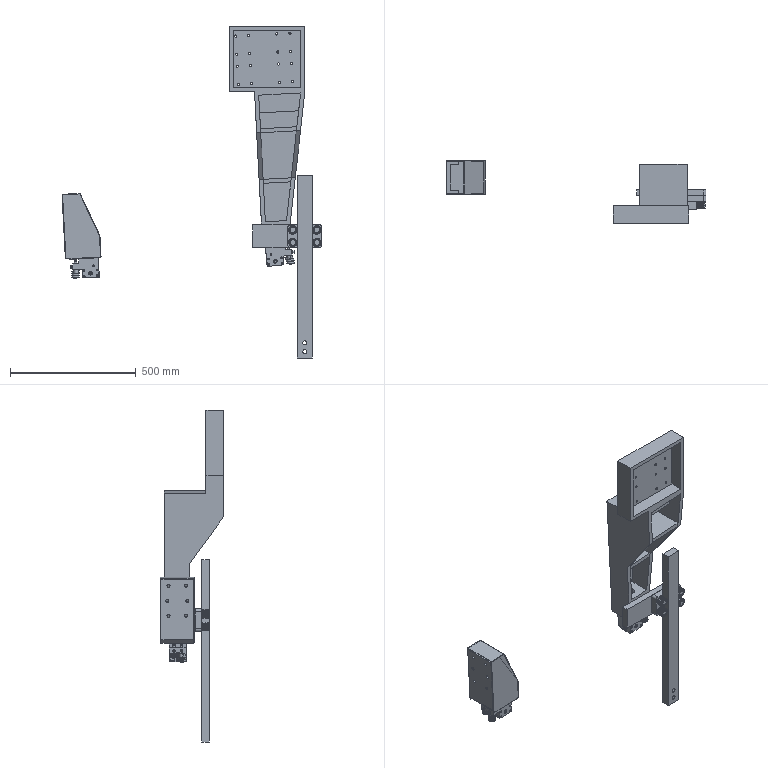Part | SolidWorks | features CompositeCurve 1 | 308 solids | 2618 faces | box 1034 x 251 x 1320 mm | volume 13536578 mm3 | plane 830 | cylinder 808 | sphere 416 | cone 336 | torus 228 | commonest cylinder face diameters 1 x72 10 x60 21.667 x48 28.333 x48 6.8 x44 8 x44